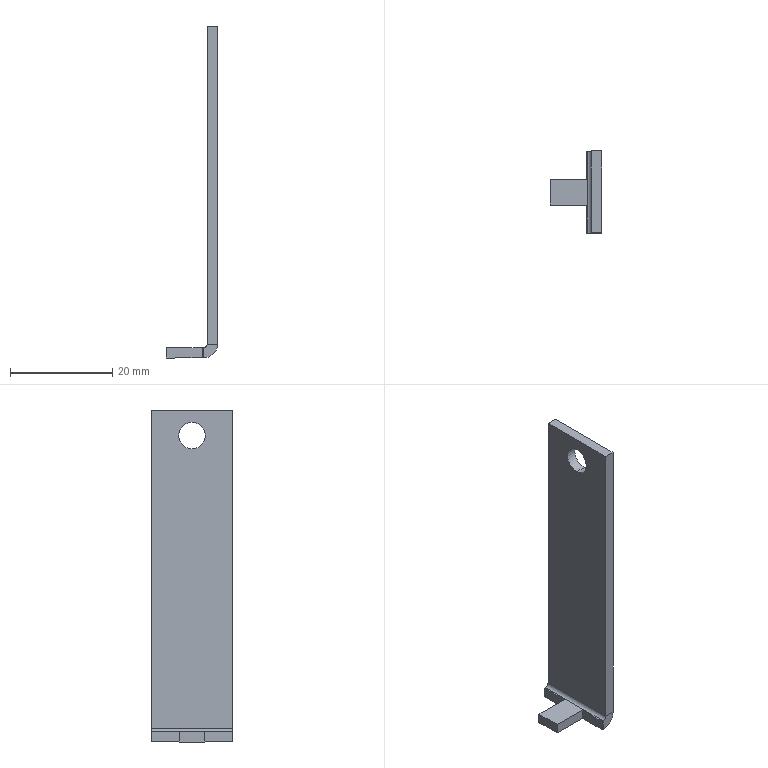Part | SolidWorks | features EdgeFlange 1, FlatPattern 1, HoleWzd 1, ICE 1, SMBaseFlange 1, SheetMetal 1 | 1 solid | 20 faces | box 10 x 16 x 65 mm | volume 2116 mm3 | plane 16 | cylinder 4 | commonest cylinder face diameters 5.2 x2 1.473 x1 5.473 x1
STEP:
#1=CARTESIAN_POINT('',(-2.,0.,30.1));
#2=VERTEX_POINT('',#1);
#3=CARTESIAN_POINT('',(-2.,0.,24.9));
#4=VERTEX_POINT('',#3);
#5=CARTESIAN_POINT('',(-2.,0.,27.5));
#6=DIRECTION('',(1.,0.,0.));
#7=DIRECTION('',(0.,0.,-1.));
#8=AXIS2_PLACEMENT_3D('',#5,#6,#7);
#9=CIRCLE('',#8,2.6);
#10=EDGE_CURVE('',#2,#4,#9,.T.);
#11=ORIENTED_EDGE('',*,*,#10,.F.);
#12=CARTESIAN_POINT('',(0.,0.,30.1));
#13=VERTEX_POINT('',#12);
#14=CARTESIAN_POINT('',(0.,0.,30.1));
#15=DIRECTION('',(1.,0.,0.));
#16=VECTOR('',#15,1000.);
#17=LINE('',#14,#16);
#18=EDGE_CURVE('',#2,#13,#17,.T.);
#19=ORIENTED_EDGE('',*,*,#18,.T.);
#20=CARTESIAN_POINT('',(0.,0.,24.9));
#21=VERTEX_POINT('',#20);
#22=CARTESIAN_POINT('',(0.,0.,27.5));
#23=DIRECTION('',(1.,0.,0.));
#24=DIRECTION('',(0.,0.,-1.));
#25=AXIS2_PLACEMENT_3D('',#22,#23,#24);
#26=CIRCLE('',#25,2.6);
#27=EDGE_CURVE('',#13,#21,#26,.T.);
#28=ORIENTED_EDGE('',*,*,#27,.T.);
#29=CARTESIAN_POINT('',(0.,0.,24.9));
#30=DIRECTION('',(1.,0.,0.));
#31=VECTOR('',#30,1000.);
#32=LINE('',#29,#31);
#33=EDGE_CURVE('',#4,#21,#32,.T.);
#34=ORIENTED_EDGE('',*,*,#33,.F.);
#35=EDGE_LOOP('',(#11,#19,#28,#34));
#36=FACE_OUTER_BOUND('',#35,.T.);
#37=CARTESIAN_POINT('',(0.,0.,27.5));
#38=DIRECTION('',(1.,0.,0.));
#39=DIRECTION('',(0.,0.,-1.));
#40=AXIS2_PLACEMENT_3D('',#37,#38,#39);
#41=CYLINDRICAL_SURFACE('',#40,2.6);
#42=ADVANCED_FACE('',(#36),#41,.F.);
#43=CARTESIAN_POINT('',(-2.,-8.,32.5));
#44=VERTEX_POINT('',#43);
#45=CARTESIAN_POINT('',(-2.,-8.,-29.763));
#46=VERTEX_POINT('',#45);
#47=CARTESIAN_POINT('',(-2.,-8.,32.5));
#48=DIRECTION('',(0.,0.,-1.));
#49=VECTOR('',#48,1000.);
#50=LINE('',#47,#49);
#51=EDGE_CURVE('',#44,#46,#50,.T.);
#52=ORIENTED_EDGE('',*,*,#51,.T.);
#53=CARTESIAN_POINT('',(0.,-8.,-29.763));
#54=VERTEX_POINT('',#53);
#55=CARTESIAN_POINT('',(-2.,-8.,-29.763));
#56=DIRECTION('',(1.,0.,0.));
#57=VECTOR('',#56,1000.);
#58=LINE('',#55,#57);
#59=EDGE_CURVE('',#46,#54,#58,.T.);
#60=ORIENTED_EDGE('',*,*,#59,.T.);
#61=CARTESIAN_POINT('',(0.,-8.,32.5));
#62=VERTEX_POINT('',#61);
#63=CARTESIAN_POINT('',(0.,-8.,32.5));
#64=DIRECTION('',(0.,0.,-1.));
#65=VECTOR('',#64,1000.);
#66=LINE('',#63,#65);
#67=EDGE_CURVE('',#62,#54,#66,.T.);
#68=ORIENTED_EDGE('',*,*,#67,.F.);
#69=CARTESIAN_POINT('',(-2.,-8.,32.5));
#70=DIRECTION('',(1.,0.,0.));
#71=VECTOR('',#70,1000.);
#72=LINE('',#69,#71);
#73=EDGE_CURVE('',#44,#62,#72,.T.);
#74=ORIENTED_EDGE('',*,*,#73,.F.);
#75=EDGE_LOOP('',(#52,#60,#68,#74));
#76=FACE_OUTER_BOUND('',#75,.T.);
#77=CARTESIAN_POINT('',(-2.,-8.,32.5));
#78=DIRECTION('',(0.,-1.,0.));
#79=DIRECTION('',(0.,0.,-1.));
#80=AXIS2_PLACEMENT_3D('',#77,#78,#79);
#81=PLANE('',#80);
#82=ADVANCED_FACE('',(#76),#81,.T.);
#83=CARTESIAN_POINT('',(-2.,0.,27.5));
#84=DIRECTION('',(1.,0.,0.));
#85=DIRECTION('',(0.,0.,-1.));
#86=AXIS2_PLACEMENT_3D('',#83,#84,#85);
#87=CIRCLE('',#86,2.6);
#88=EDGE_CURVE('',#4,#2,#87,.T.);
#89=ORIENTED_EDGE('',*,*,#88,.T.);
#90=ORIENTED_EDGE('',*,*,#10,.T.);
#91=EDGE_LOOP('',(#89,#90));
#92=FACE_BOUND('',#91,.T.);
#93=CARTESIAN_POINT('',(-2.,8.,-29.763));
#94=VERTEX_POINT('',#93);
#95=CARTESIAN_POINT('',(-2.,-8.,-29.763));
#96=DIRECTION('',(0.,1.,0.));
#97=VECTOR('',#96,1000.);
#98=LINE('',#95,#97);
#99=EDGE_CURVE('',#46,#94,#98,.T.);
#100=ORIENTED_EDGE('',*,*,#99,.F.);
#101=ORIENTED_EDGE('',*,*,#51,.F.);
#102=CARTESIAN_POINT('',(-2.,8.,32.5));
#103=VERTEX_POINT('',#102);
#104=CARTESIAN_POINT('',(-2.,8.,32.5));
#105=DIRECTION('',(0.,-1.,0.));
#106=VECTOR('',#105,1000.);
#107=LINE('',#104,#106);
#108=EDGE_CURVE('',#103,#44,#107,.T.);
#109=ORIENTED_EDGE('',*,*,#108,.F.);
#110=CARTESIAN_POINT('',(-2.,8.,32.5));
#111=DIRECTION('',(0.,0.,1.));
#112=VECTOR('',#111,1000.);
#113=LINE('',#110,#112);
#114=EDGE_CURVE('',#94,#103,#113,.T.);
#115=ORIENTED_EDGE('',*,*,#114,.F.);
#116=EDGE_LOOP('',(#100,#101,#109,#115));
#117=FACE_OUTER_BOUND('',#116,.T.);
#118=CARTESIAN_POINT('',(-2.,0.,0.));
#119=DIRECTION('',(1.,0.,0.));
#120=DIRECTION('',(0.,0.,-1.));
#121=AXIS2_PLACEMENT_3D('',#118,#119,#120);
#122=PLANE('',#121);
#123=ADVANCED_FACE('',(#92,#117),#122,.F.);
#124=CARTESIAN_POINT('',(0.,0.,27.5));
#125=DIRECTION('',(1.,0.,0.));
#126=DIRECTION('',(0.,0.,-1.));
#127=AXIS2_PLACEMENT_3D('',#124,#125,#126);
#128=CIRCLE('',#127,2.6);
#129=EDGE_CURVE('',#21,#13,#128,.T.);
#130=ORIENTED_EDGE('',*,*,#129,.F.);
#131=ORIENTED_EDGE('',*,*,#27,.F.);
#132=EDGE_LOOP('',(#130,#131));
#133=FACE_BOUND('',#132,.T.);
#134=ORIENTED_EDGE('',*,*,#67,.T.);
#135=CARTESIAN_POINT('',(0.,8.,-29.763));
#136=VERTEX_POINT('',#135);
#137=CARTESIAN_POINT('',(0.,-8.,-29.763));
#138=DIRECTION('',(0.,1.,0.));
#139=VECTOR('',#138,1000.);
#140=LINE('',#137,#139);
#141=EDGE_CURVE('',#54,#136,#140,.T.);
#142=ORIENTED_EDGE('',*,*,#141,.T.);
#143=CARTESIAN_POINT('',(0.,8.,32.5));
#144=VERTEX_POINT('',#143);
#145=CARTESIAN_POINT('',(0.,8.,32.5));
#146=DIRECTION('',(0.,0.,1.));
#147=VECTOR('',#146,1000.);
#148=LINE('',#145,#147);
#149=EDGE_CURVE('',#136,#144,#148,.T.);
#150=ORIENTED_EDGE('',*,*,#149,.T.);
#151=CARTESIAN_POINT('',(0.,8.,32.5));
#152=DIRECTION('',(0.,-1.,0.));
#153=VECTOR('',#152,1000.);
#154=LINE('',#151,#153);
#155=EDGE_CURVE('',#144,#62,#154,.T.);
#156=ORIENTED_EDGE('',*,*,#155,.T.);
#157=EDGE_LOOP('',(#134,#142,#150,#156));
#158=FACE_OUTER_BOUND('',#157,.T.);
#159=CARTESIAN_POINT('',(0.,0.,0.));
#160=DIRECTION('',(1.,0.,0.));
#161=DIRECTION('',(0.,0.,-1.));
#162=AXIS2_PLACEMENT_3D('',#159,#160,#161);
#163=PLANE('',#162);
#164=ADVANCED_FACE('',(#133,#158),#163,.T.);
#165=ORIENTED_EDGE('',*,*,#155,.F.);
#166=CARTESIAN_POINT('',(-2.,8.,32.5));
#167=DIRECTION('',(1.,0.,0.));
#168=VECTOR('',#167,1000.);
#169=LINE('',#166,#168);
#170=EDGE_CURVE('',#103,#144,#169,.T.);
#171=ORIENTED_EDGE('',*,*,#170,.F.);
#172=ORIENTED_EDGE('',*,*,#108,.T.);
#173=ORIENTED_EDGE('',*,*,#73,.T.);
#174=EDGE_LOOP('',(#165,#171,#172,#173));
#175=FACE_OUTER_BOUND('',#174,.T.);
#176=CARTESIAN_POINT('',(-2.,8.,32.5));
#177=DIRECTION('',(0.,0.,1.));
#178=DIRECTION('',(1.,0.,0.));
#179=AXIS2_PLACEMENT_3D('',#176,#177,#178);
#180=PLANE('',#179);
#181=ADVANCED_FACE('',(#175),#180,.T.);
#182=CARTESIAN_POINT('',(-2.,8.,-29.763));
#183=DIRECTION('',(1.,0.,0.));
#184=VECTOR('',#183,1000.);
#185=LINE('',#182,#184);
#186=EDGE_CURVE('',#94,#136,#185,.T.);
#187=ORIENTED_EDGE('',*,*,#186,.F.);
#188=ORIENTED_EDGE('',*,*,#114,.T.);
#189=ORIENTED_EDGE('',*,*,#170,.T.);
#190=ORIENTED_EDGE('',*,*,#149,.F.);
#191=EDGE_LOOP('',(#187,#188,#189,#190));
#192=FACE_OUTER_BOUND('',#191,.T.);
#193=CARTESIAN_POINT('',(-2.,8.,32.5));
#194=DIRECTION('',(0.,1.,0.));
#195=DIRECTION('',(0.,0.,1.));
#196=AXIS2_PLACEMENT_3D('',#193,#194,#195);
#197=PLANE('',#196);
#198=ADVANCED_FACE('',(#192),#197,.T.);
#199=CARTESIAN_POINT('',(-2.737,8.,-30.5));
#200=VERTEX_POINT('',#199);
#201=CARTESIAN_POINT('',(-2.737,8.,-32.5));
#202=VERTEX_POINT('',#201);
#203=CARTESIAN_POINT('',(-2.737,8.,-32.5));
#204=DIRECTION('',(0.,0.,-1.));
#205=VECTOR('',#204,1000.);
#206=LINE('',#203,#205);
#207=EDGE_CURVE('',#200,#202,#206,.T.);
#208=ORIENTED_EDGE('',*,*,#207,.F.);
#209=CARTESIAN_POINT('',(-2.737,8.,-29.763));
#210=DIRECTION('',(0.,1.,0.));
#211=DIRECTION('',(0.,0.,-1.));
#212=AXIS2_PLACEMENT_3D('',#209,#210,#211);
#213=CIRCLE('',#212,0.7366);
#214=EDGE_CURVE('',#94,#200,#213,.T.);
#215=ORIENTED_EDGE('',*,*,#214,.F.);
#216=ORIENTED_EDGE('',*,*,#186,.T.);
#217=CARTESIAN_POINT('',(-2.737,8.,-29.763));
#218=DIRECTION('',(0.,1.,0.));
#219=DIRECTION('',(0.,0.,-1.));
#220=AXIS2_PLACEMENT_3D('',#217,#218,#219);
#221=CIRCLE('',#220,2.737);
#222=EDGE_CURVE('',#136,#202,#221,.T.);
#223=ORIENTED_EDGE('',*,*,#222,.T.);
#224=EDGE_LOOP('',(#208,#215,#216,#223));
#225=FACE_OUTER_BOUND('',#224,.T.);
#226=CARTESIAN_POINT('',(-2.737,8.,-29.763));
#227=DIRECTION('',(0.,1.,0.));
#228=DIRECTION('',(0.,0.,1.));
#229=AXIS2_PLACEMENT_3D('',#226,#227,#228);
#230=PLANE('',#229);
#231=ADVANCED_FACE('',(#225),#230,.T.);
#232=CARTESIAN_POINT('',(-2.737,-8.,-30.5));
#233=VERTEX_POINT('',#232);
#234=CARTESIAN_POINT('',(-2.737,-8.,-29.763));
#235=DIRECTION('',(0.,-1.,0.));
#236=DIRECTION('',(0.,0.,-1.));
#237=AXIS2_PLACEMENT_3D('',#234,#235,#236);
#238=CIRCLE('',#237,0.7366);
#239=EDGE_CURVE('',#233,#46,#238,.T.);
#240=ORIENTED_EDGE('',*,*,#239,.F.);
#241=CARTESIAN_POINT('',(-2.737,-8.,-32.5));
#242=VERTEX_POINT('',#241);
#243=CARTESIAN_POINT('',(-2.737,-8.,-30.5));
#244=DIRECTION('',(0.,0.,-1.));
#245=VECTOR('',#244,1000.);
#246=LINE('',#243,#245);
#247=EDGE_CURVE('',#233,#242,#246,.T.);
#248=ORIENTED_EDGE('',*,*,#247,.T.);
#249=CARTESIAN_POINT('',(-2.737,-8.,-29.763));
#250=DIRECTION('',(0.,-1.,0.));
#251=DIRECTION('',(0.,0.,-1.));
#252=AXIS2_PLACEMENT_3D('',#249,#250,#251);
#253=CIRCLE('',#252,2.737);
#254=EDGE_CURVE('',#242,#54,#253,.T.);
#255=ORIENTED_EDGE('',*,*,#254,.T.);
#256=ORIENTED_EDGE('',*,*,#59,.F.);
#257=EDGE_LOOP('',(#240,#248,#255,#256));
#258=FACE_OUTER_BOUND('',#257,.T.);
#259=CARTESIAN_POINT('',(-2.737,-8.,-29.763));
#260=DIRECTION('',(0.,1.,0.));
#261=DIRECTION('',(0.,0.,1.));
#262=AXIS2_PLACEMENT_3D('',#259,#260,#261);
#263=PLANE('',#262);
#264=ADVANCED_FACE('',(#258),#263,.F.);
#265=ORIENTED_EDGE('',*,*,#141,.F.);
#266=ORIENTED_EDGE('',*,*,#254,.F.);
#267=CARTESIAN_POINT('',(-2.737,8.,-32.5));
#268=DIRECTION('',(0.,1.,0.));
#269=VECTOR('',#268,1000.);
#270=LINE('',#267,#269);
#271=EDGE_CURVE('',#242,#202,#270,.T.);
#272=ORIENTED_EDGE('',*,*,#271,.T.);
#273=ORIENTED_EDGE('',*,*,#222,.F.);
#274=EDGE_LOOP('',(#265,#266,#272,#273));
#275=FACE_OUTER_BOUND('',#274,.T.);
#276=CARTESIAN_POINT('',(-2.737,-8.,-29.763));
#277=DIRECTION('',(0.,-1.,0.));
#278=DIRECTION('',(0.,0.,-1.));
#279=AXIS2_PLACEMENT_3D('',#276,#277,#278);
#280=CYLINDRICAL_SURFACE('',#279,2.737);
#281=ADVANCED_FACE('',(#275),#280,.T.);
#282=ORIENTED_EDGE('',*,*,#99,.T.);
#283=ORIENTED_EDGE('',*,*,#214,.T.);
#284=CARTESIAN_POINT('',(-2.737,8.,-30.5));
#285=DIRECTION('',(0.,-1.,0.));
#286=VECTOR('',#285,1000.);
#287=LINE('',#284,#286);
#288=EDGE_CURVE('',#200,#233,#287,.T.);
#289=ORIENTED_EDGE('',*,*,#288,.T.);
#290=ORIENTED_EDGE('',*,*,#239,.T.);
#291=EDGE_LOOP('',(#282,#283,#289,#290));
#292=FACE_OUTER_BOUND('',#291,.T.);
#293=CARTESIAN_POINT('',(-2.737,-8.,-29.763));
#294=DIRECTION('',(0.,-1.,0.));
#295=DIRECTION('',(0.,0.,-1.));
#296=AXIS2_PLACEMENT_3D('',#293,#294,#295);
#297=CYLINDRICAL_SURFACE('',#296,0.7366);
#298=ADVANCED_FACE('',(#292),#297,.F.);
#299=CARTESIAN_POINT('',(-3.,-8.,-30.5));
#300=VERTEX_POINT('',#299);
#301=CARTESIAN_POINT('',(-10.,-8.,-30.5));
#302=DIRECTION('',(-1.,0.,0.));
#303=VECTOR('',#302,1000.);
#304=LINE('',#301,#303);
#305=EDGE_CURVE('',#233,#300,#304,.T.);
#306=ORIENTED_EDGE('',*,*,#305,.T.);
#307=CARTESIAN_POINT('',(-3.,-8.,-32.5));
#308=VERTEX_POINT('',#307);
#309=CARTESIAN_POINT('',(-3.,-8.,-32.5));
#310=DIRECTION('',(0.,0.,-1.));
#311=VECTOR('',#310,1000.);
#312=LINE('',#309,#311);
#313=EDGE_CURVE('',#300,#308,#312,.T.);
#314=ORIENTED_EDGE('',*,*,#313,.T.);
#315=CARTESIAN_POINT('',(0.,-8.,-32.5));
#316=DIRECTION('',(-1.,0.,0.));
#317=VECTOR('',#316,1000.);
#318=LINE('',#315,#317);
#319=EDGE_CURVE('',#242,#308,#318,.T.);
#320=ORIENTED_EDGE('',*,*,#319,.F.);
#321=ORIENTED_EDGE('',*,*,#247,.F.);
#322=EDGE_LOOP('',(#306,#314,#320,#321));
#323=FACE_OUTER_BOUND('',#322,.T.);
#324=CARTESIAN_POINT('',(-10.,-8.,-32.5));
#325=DIRECTION('',(0.,1.,0.));
#326=DIRECTION('',(-1.,0.,0.));
#327=AXIS2_PLACEMENT_3D('',#324,#325,#326);
#328=PLANE('',#327);
#329=ADVANCED_FACE('',(#323),#328,.F.);
#330=CARTESIAN_POINT('',(-3.,8.,-32.5));
#331=VERTEX_POINT('',#330);
#332=CARTESIAN_POINT('',(0.,8.,-32.5));
#333=DIRECTION('',(1.,0.,0.));
#334=VECTOR('',#333,1000.);
#335=LINE('',#332,#334);
#336=EDGE_CURVE('',#331,#202,#335,.T.);
#337=ORIENTED_EDGE('',*,*,#336,.F.);
#338=CARTESIAN_POINT('',(-3.,8.,-30.5));
#339=VERTEX_POINT('',#338);
#340=CARTESIAN_POINT('',(-3.,8.,-32.5));
#341=DIRECTION('',(0.,0.,1.));
#342=VECTOR('',#341,1000.);
#343=LINE('',#340,#342);
#344=EDGE_CURVE('',#331,#339,#343,.T.);
#345=ORIENTED_EDGE('',*,*,#344,.T.);
#346=CARTESIAN_POINT('',(-2.,8.,-30.5));
#347=DIRECTION('',(1.,0.,0.));
#348=VECTOR('',#347,1000.);
#349=LINE('',#346,#348);
#350=EDGE_CURVE('',#339,#200,#349,.T.);
#351=ORIENTED_EDGE('',*,*,#350,.T.);
#352=ORIENTED_EDGE('',*,*,#207,.T.);
#353=EDGE_LOOP('',(#337,#345,#351,#352));
#354=FACE_OUTER_BOUND('',#353,.T.);
#355=CARTESIAN_POINT('',(-2.,8.,-32.5));
#356=DIRECTION('',(0.,-1.,0.));
#357=DIRECTION('',(1.,0.,0.));
#358=AXIS2_PLACEMENT_3D('',#355,#356,#357);
#359=PLANE('',#358);
#360=ADVANCED_FACE('',(#354),#359,.F.);
#361=CARTESIAN_POINT('',(-10.,-2.5,-32.5));
#362=VERTEX_POINT('',#361);
#363=CARTESIAN_POINT('',(-10.,2.5,-32.5));
#364=VERTEX_POINT('',#363);
#365=CARTESIAN_POINT('',(-10.,0.,-32.5));
#366=DIRECTION('',(0.,1.,0.));
#367=VECTOR('',#366,1000.);
#368=LINE('',#365,#367);
#369=EDGE_CURVE('',#362,#364,#368,.T.);
#370=ORIENTED_EDGE('',*,*,#369,.T.);
#371=CARTESIAN_POINT('',(-3.,2.5,-32.5));
#372=VERTEX_POINT('',#371);
#373=CARTESIAN_POINT('',(-10.,2.5,-32.5));
#374=DIRECTION('',(-1.,0.,0.));
#375=VECTOR('',#374,1000.);
#376=LINE('',#373,#375);
#377=EDGE_CURVE('',#372,#364,#376,.T.);
#378=ORIENTED_EDGE('',*,*,#377,.F.);
#379=CARTESIAN_POINT('',(-3.,2.5,-32.5));
#380=DIRECTION('',(0.,-1.,0.));
#381=VECTOR('',#380,1000.);
#382=LINE('',#379,#381);
#383=EDGE_CURVE('',#331,#372,#382,.T.);
#384=ORIENTED_EDGE('',*,*,#383,.F.);
#385=ORIENTED_EDGE('',*,*,#336,.T.);
#386=ORIENTED_EDGE('',*,*,#271,.F.);
#387=ORIENTED_EDGE('',*,*,#319,.T.);
#388=CARTESIAN_POINT('',(-3.,-2.5,-32.5));
#389=VERTEX_POINT('',#388);
#390=CARTESIAN_POINT('',(-3.,-2.5,-32.5));
#391=DIRECTION('',(0.,-1.,0.));
#392=VECTOR('',#391,1000.);
#393=LINE('',#390,#392);
#394=EDGE_CURVE('',#389,#308,#393,.T.);
#395=ORIENTED_EDGE('',*,*,#394,.F.);
#396=CARTESIAN_POINT('',(-10.,-2.5,-32.5));
#397=DIRECTION('',(1.,0.,0.));
#398=VECTOR('',#397,1000.);
#399=LINE('',#396,#398);
#400=EDGE_CURVE('',#362,#389,#399,.T.);
#401=ORIENTED_EDGE('',*,*,#400,.F.);
#402=EDGE_LOOP('',(#370,#378,#384,#385,#386,#387,#395,#401));
#403=FACE_OUTER_BOUND('',#402,.T.);
#404=CARTESIAN_POINT('',(0.,0.,-32.5));
#405=DIRECTION('',(0.,0.,1.));
#406=DIRECTION('',(1.,0.,0.));
#407=AXIS2_PLACEMENT_3D('',#404,#405,#406);
#408=PLANE('',#407);
#409=ADVANCED_FACE('',(#403),#408,.F.);
#410=CARTESIAN_POINT('',(-10.,2.5,-30.5));
#411=VERTEX_POINT('',#410);
#412=CARTESIAN_POINT('',(-3.,2.5,-30.5));
#413=VERTEX_POINT('',#412);
#414=CARTESIAN_POINT('',(0.,2.5,-30.5));
#415=DIRECTION('',(1.,0.,0.));
#416=VECTOR('',#415,1000.);
#417=LINE('',#414,#416);
#418=EDGE_CURVE('',#411,#413,#417,.T.);
#419=ORIENTED_EDGE('',*,*,#418,.F.);
#420=CARTESIAN_POINT('',(-10.,-2.5,-30.5));
#421=VERTEX_POINT('',#420);
#422=CARTESIAN_POINT('',(-10.,8.,-30.5));
#423=DIRECTION('',(0.,1.,0.));
#424=VECTOR('',#423,1000.);
#425=LINE('',#422,#424);
#426=EDGE_CURVE('',#421,#411,#425,.T.);
#427=ORIENTED_EDGE('',*,*,#426,.F.);
#428=CARTESIAN_POINT('',(-3.,-2.5,-30.5));
#429=VERTEX_POINT('',#428);
#430=CARTESIAN_POINT('',(0.,-2.5,-30.5));
#431=DIRECTION('',(-1.,0.,0.));
#432=VECTOR('',#431,1000.);
#433=LINE('',#430,#432);
#434=EDGE_CURVE('',#429,#421,#433,.T.);
#435=ORIENTED_EDGE('',*,*,#434,.F.);
#436=CARTESIAN_POINT('',(-3.,0.,-30.5));
#437=DIRECTION('',(0.,1.,0.));
#438=VECTOR('',#437,1000.);
#439=LINE('',#436,#438);
#440=EDGE_CURVE('',#300,#429,#439,.T.);
#441=ORIENTED_EDGE('',*,*,#440,.F.);
#442=ORIENTED_EDGE('',*,*,#305,.F.);
#443=ORIENTED_EDGE('',*,*,#288,.F.);
#444=ORIENTED_EDGE('',*,*,#350,.F.);
#445=CARTESIAN_POINT('',(-3.,0.,-30.5));
#446=DIRECTION('',(0.,1.,0.));
#447=VECTOR('',#446,1000.);
#448=LINE('',#445,#447);
#449=EDGE_CURVE('',#413,#339,#448,.T.);
#450=ORIENTED_EDGE('',*,*,#449,.F.);
#451=EDGE_LOOP('',(#419,#427,#435,#441,#442,#443,#444,#450));
#452=FACE_OUTER_BOUND('',#451,.T.);
#453=CARTESIAN_POINT('',(0.,0.,-30.5));
#454=DIRECTION('',(0.,0.,1.));
#455=DIRECTION('',(1.,0.,0.));
#456=AXIS2_PLACEMENT_3D('',#453,#454,#455);
#457=PLANE('',#456);
#458=ADVANCED_FACE('',(#452),#457,.T.);
#459=ORIENTED_EDGE('',*,*,#426,.T.);
#460=CARTESIAN_POINT('',(-10.,2.5,-32.5));
#461=DIRECTION('',(0.,0.,-1.));
#462=VECTOR('',#461,1000.);
#463=LINE('',#460,#462);
#464=EDGE_CURVE('',#411,#364,#463,.T.);
#465=ORIENTED_EDGE('',*,*,#464,.T.);
#466=ORIENTED_EDGE('',*,*,#369,.F.);
#467=CARTESIAN_POINT('',(-10.,-2.5,-32.5));
#468=DIRECTION('',(0.,0.,1.));
#469=VECTOR('',#468,1000.);
#470=LINE('',#467,#469);
#471=EDGE_CURVE('',#362,#421,#470,.T.);
#472=ORIENTED_EDGE('',*,*,#471,.T.);
#473=EDGE_LOOP('',(#459,#465,#466,#472));
#474=FACE_OUTER_BOUND('',#473,.T.);
#475=CARTESIAN_POINT('',(-10.,8.,-32.5));
#476=DIRECTION('',(1.,0.,0.));
#477=DIRECTION('',(0.,0.,-1.));
#478=AXIS2_PLACEMENT_3D('',#475,#476,#477);
#479=PLANE('',#478);
#480=ADVANCED_FACE('',(#474),#479,.F.);
#481=ORIENTED_EDGE('',*,*,#434,.T.);
#482=ORIENTED_EDGE('',*,*,#471,.F.);
#483=ORIENTED_EDGE('',*,*,#400,.T.);
#484=CARTESIAN_POINT('',(-3.,-2.5,32.5));
#485=DIRECTION('',(0.,0.,-1.));
#486=VECTOR('',#485,1000.);
#487=LINE('',#484,#486);
#488=EDGE_CURVE('',#429,#389,#487,.T.);
#489=ORIENTED_EDGE('',*,*,#488,.F.);
#490=EDGE_LOOP('',(#481,#482,#483,#489));
#491=FACE_OUTER_BOUND('',#490,.T.);
#492=CARTESIAN_POINT('',(-10.,-2.5,32.5));
#493=DIRECTION('',(0.,1.,0.));
#494=DIRECTION('',(-1.,0.,0.));
#495=AXIS2_PLACEMENT_3D('',#492,#493,#494);
#496=PLANE('',#495);
#497=ADVANCED_FACE('',(#491),#496,.F.);
#498=ORIENTED_EDGE('',*,*,#440,.T.);
#499=ORIENTED_EDGE('',*,*,#488,.T.);
#500=ORIENTED_EDGE('',*,*,#394,.T.);
#501=ORIENTED_EDGE('',*,*,#313,.F.);
#502=EDGE_LOOP('',(#498,#499,#500,#501));
#503=FACE_OUTER_BOUND('',#502,.T.);
#504=CARTESIAN_POINT('',(-3.,-2.5,32.5));
#505=DIRECTION('',(1.,0.,0.));
#506=DIRECTION('',(0.,0.,-1.));
#507=AXIS2_PLACEMENT_3D('',#504,#505,#506);
#508=PLANE('',#507);
#509=ADVANCED_FACE('',(#503),#508,.F.);
#510=ORIENTED_EDGE('',*,*,#383,.T.);
#511=CARTESIAN_POINT('',(-3.,2.5,32.5));
#512=DIRECTION('',(0.,0.,-1.));
#513=VECTOR('',#512,1000.);
#514=LINE('',#511,#513);
#515=EDGE_CURVE('',#413,#372,#514,.T.);
#516=ORIENTED_EDGE('',*,*,#515,.F.);
#517=ORIENTED_EDGE('',*,*,#449,.T.);
#518=ORIENTED_EDGE('',*,*,#344,.F.);
#519=EDGE_LOOP('',(#510,#516,#517,#518));
#520=FACE_OUTER_BOUND('',#519,.T.);
#521=CARTESIAN_POINT('',(-3.,2.5,32.5));
#522=DIRECTION('',(1.,0.,0.));
#523=DIRECTION('',(0.,0.,-1.));
#524=AXIS2_PLACEMENT_3D('',#521,#522,#523);
#525=PLANE('',#524);
#526=ADVANCED_FACE('',(#520),#525,.F.);
#527=ORIENTED_EDGE('',*,*,#418,.T.);
#528=ORIENTED_EDGE('',*,*,#515,.T.);
#529=ORIENTED_EDGE('',*,*,#377,.T.);
#530=ORIENTED_EDGE('',*,*,#464,.F.);
#531=EDGE_LOOP('',(#527,#528,#529,#530));
#532=FACE_OUTER_BOUND('',#531,.T.);
#533=CARTESIAN_POINT('',(-10.,2.5,32.5));
#534=DIRECTION('',(0.,-1.,0.));
#535=DIRECTION('',(1.,0.,0.));
#536=AXIS2_PLACEMENT_3D('',#533,#534,#535);
#537=PLANE('',#536);
#538=ADVANCED_FACE('',(#532),#537,.F.);
#539=ORIENTED_EDGE('',*,*,#18,.F.);
#540=ORIENTED_EDGE('',*,*,#88,.F.);
#541=ORIENTED_EDGE('',*,*,#33,.T.);
#542=ORIENTED_EDGE('',*,*,#129,.T.);
#543=EDGE_LOOP('',(#539,#540,#541,#542));
#544=FACE_OUTER_BOUND('',#543,.T.);
#545=CARTESIAN_POINT('',(0.,0.,27.5));
#546=DIRECTION('',(1.,0.,0.));
#547=DIRECTION('',(0.,0.,-1.));
#548=AXIS2_PLACEMENT_3D('',#545,#546,#547);
#549=CYLINDRICAL_SURFACE('',#548,2.6);
#550=ADVANCED_FACE('',(#544),#549,.F.);
#551=CLOSED_SHELL('',(#42,#82,#123,#164,#181,#198,#231,#264,#281,#298,#329,#360,#409,#458,#480,#497,#509,#526,#538,#550));
#552=MANIFOLD_SOLID_BREP('',#551);
#553=CARTESIAN_POINT('',(0.,0.,0.));
#554=DIRECTION('',(0.,0.,1.));
#555=DIRECTION('',(1.,0.,0.));
#556=AXIS2_PLACEMENT_3D('',#553,#554,#555);
#557=(LENGTH_UNIT()NAMED_UNIT(*)SI_UNIT(.MILLI.,.METRE.));
#558=UNCERTAINTY_MEASURE_WITH_UNIT(LENGTH_MEASURE(0.00001),#557,'','');
#559=(NAMED_UNIT(*)PLANE_ANGLE_UNIT()SI_UNIT($,.RADIAN.));
#560=(NAMED_UNIT(*)SI_UNIT($,.STERADIAN.)SOLID_ANGLE_UNIT());
#561=(GEOMETRIC_REPRESENTATION_CONTEXT(3)GLOBAL_UNCERTAINTY_ASSIGNED_CONTEXT((#558))GLOBAL_UNIT_ASSIGNED_CONTEXT((#557,#559,#560))REPRESENTATION_CONTEXT('',''));
#562=ADVANCED_BREP_SHAPE_REPRESENTATION('',(#552,#556),#561);